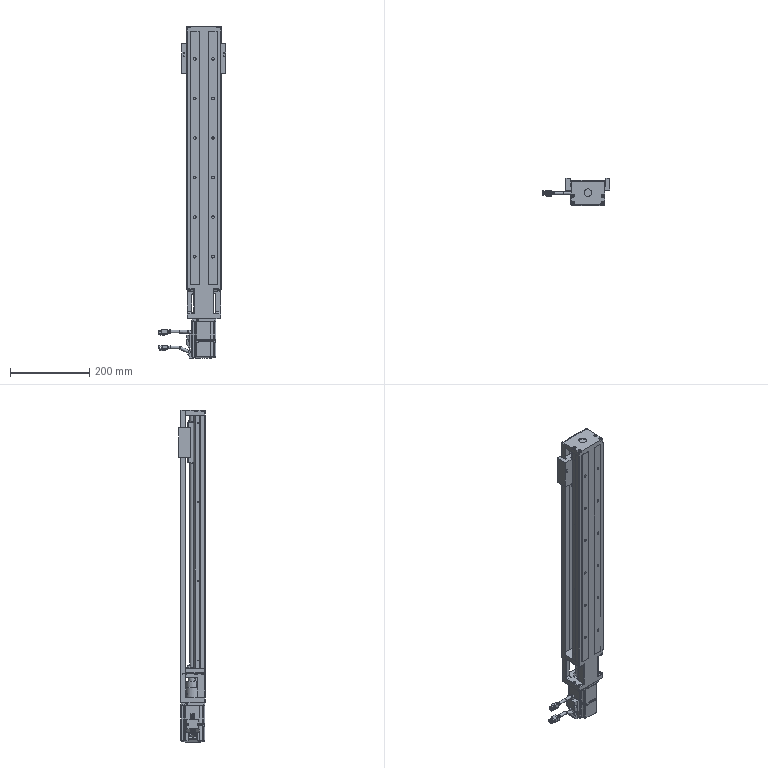Part | NX | 12 solids | 1286 faces | box 171.8 x 68 x 839 mm | volume 2074942 mm3 | plane 867 | cylinder 349 | cone 41 | spline 29 | commonest cylinder face diameters 4 x50 3 x31 8 x31 6 x30 0.6 x18 6.5 x18